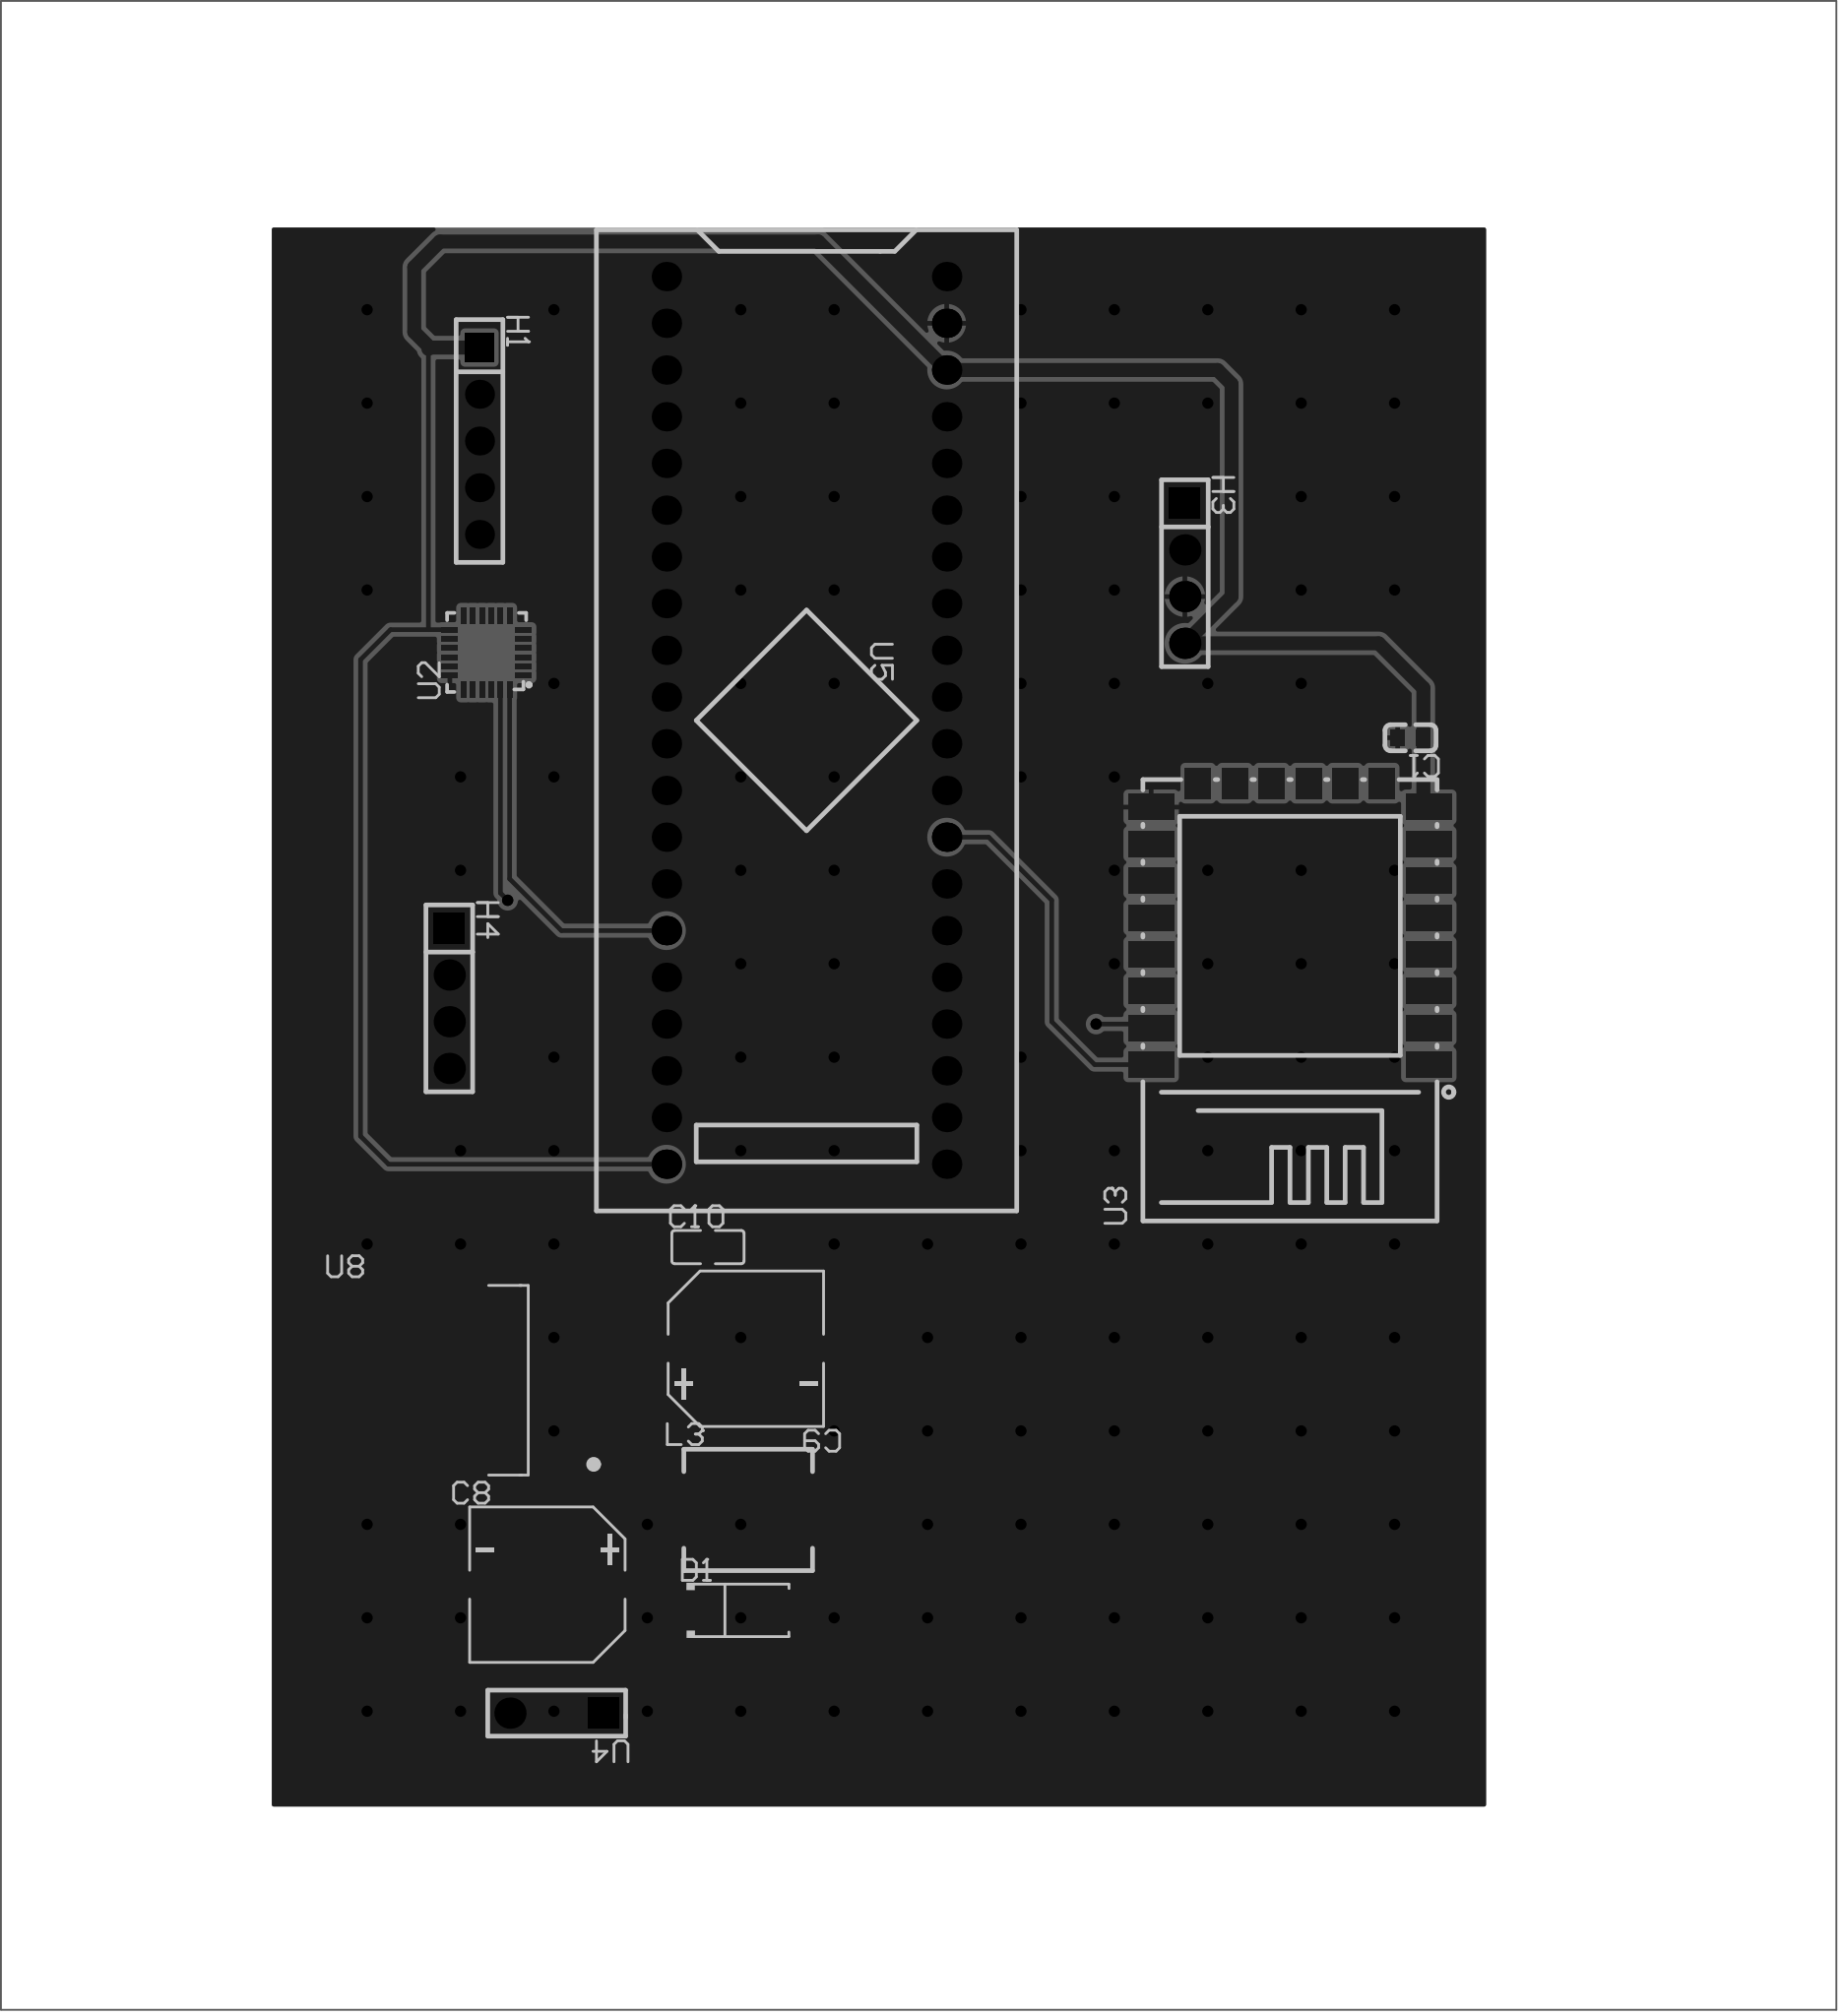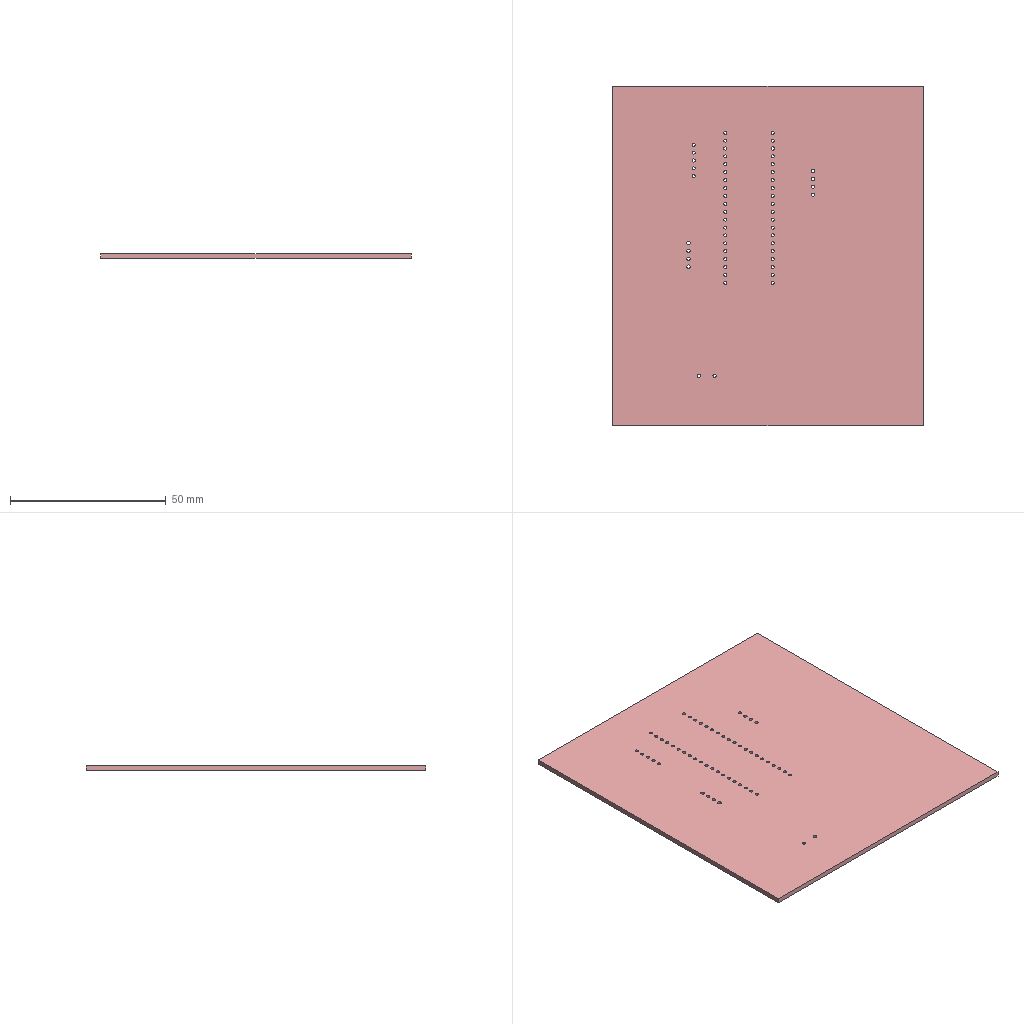Circuit board layout | Altium Designer | box 99.8 x 109.2 x 1.6 mm
Layer stack:
# Altium Designer layer stack of  (unit mm; dielectric type: 0 none, 1 core, 2 prepreg, 3 surface material)
index,name,kind,layer,copper_thickness_mm,dielectric_type,dielectric_thickness_mm,dielectric_material,dielectric_constant
0,Top Paste Mask Layer,other,,,,,,
1,Top Silkscreen Layer,other,,,,,,
2,Top Solder Mask Layer,dielectric,,,3,0.01,,3.3
3,Top Layer,copper,Top Layer,0.035,,,,
4,Dielectric1,dielectric,,,3,1.51,FR4,4.5
5,Bottom Layer,copper,Bottom Layer,0.035,,,,
6,Bottom Solder Mask Layer,dielectric,,,3,0.01,,3.3
7,Bottom Silkscreen Layer,other,,,,,,
8,Bottom Paste Mask Layer,other,,,,,,
# drill layer pairs: low layer,high layer
drill_pair,Top Layer,Bottom Layer
Part placement:
Designator,Comment,Layer,Footprint,Center-X(mm),Center-Y(mm),Rotation
C8,,TopLayer,CAP-SMD_BD8.0-L8.3-W8.3-RD,99.568,92.964,0
C9,,TopLayer,CAP-SMD_BD8.0-L8.3-W8.3-RD,110.363,105.791,180
C10,,TopLayer,C0805,108.302,111.317,0
D1,,TopLayer,SMA_L4.3-W2.6-LS5.2-RD,110.109,91.567,0
H3,Encoder,TopLayer,HDR-TH_4P-P2.54-V-M,134.239,147.955,270
H4,Servo,TopLayer,HDR-TH_4P-P2.54-V-M,94.234,124.841,270
L3,,TopLayer,IND-SMD_L7.0-W6.6,110.49,97.028,0
U2,MPU6050,TopLayer,QFN-24_L4.0-W4.0-P0.50-BL,96.266,143.637,90
U3,ESP8266,TopLayer,WIFIM-SMD_ESP-12F-ESP8266MOD,139.955,128.89,90
U4,5.08-2PIN straight header,TopLayer,HDR-TH_2P-P5.08_C9900004333,100.076,85.979,180
U8,LM2596S-5.0,TopLayer,TO-263-5_L10.2-W8.9-P1.70-BR,97.029,104.078,0
C1,10uF,TopLayer,C0603,146.511,139.01,180
U5,STM32F103C8T6-Card,TopLayer,CONN-TH_L53.3-W22.9_STM32F103C8T6-CARD,113.665,139.954,270
H1,,TopLayer,HDR-TH_5P-P2.54-V-F,95.879,155.144,270
Pad and via stacks:
# Altium Designer via and pad stacks of  (unit mm). Each distinct definition once, with the count of objects using it.
# via: kind,start_layer,end_layer,hole_mm,diameter_mm,mode(0 simple;1 top-mid-bottom;2 full stack),diameter_per_layer,count,example_net
# pad: kind,layer,hole_mm,hole_type(0 round;1 square;2 slot),plating,top_size,top_shape(1 round;2 rect;3 octagon;9 rounded rect),mid_size,bottom_size,mode,footprint,size_per_layer,count,example
pad,Top Layer,0,0,plated,3.61x1.26,2,3.61x1.26,3.61x1.26,0,CAP-SMD_BD8.0-L8.3-W8.3-RD,,4,C8.1
pad,Top Layer,0,0,plated,1.41x1.35,2,1.41x1.35,1.41x1.35,0,C0805,,2,C10.2
pad,Top Layer,0,0,plated,2x2,2,2x2,2x2,0,SMA_L4.3-W2.6-LS5.2-RD,,2,D1.2
pad,Top Layer,0,0,plated,2.799x3.701,2,2.799x3.701,2.799x3.701,0,IND-SMD_L7.0-W6.6,,2,L3.1
pad,Top Layer,0,0,plated,0.3x0.9,2,0.3x0.9,0.3x0.9,0,QFN-24_L4.0-W4.0-P0.50-BL,,24,U2.1
pad,Top Layer,0,0,plated,2.5x1.4,2,2.5x1.4,2.5x1.4,0,WIFIM-SMD_ESP-12F-ESP8266MOD,,16,U3.16
pad,Top Layer,0,0,plated,1.7x1.4,2,1.7x1.4,1.7x1.4,0,WIFIM-SMD_ESP-12F-ESP8266MOD,,6,U3.22
pad,Top Layer,0,0,plated,3.083x1.02,2,3.083x1.02,3.083x1.02,0,TO-263-5_L10.2-W8.9-P1.70-BR,,5,U8.1
pad,Top Layer,0,0,plated,8.5x11,2,8.5x11,8.5x11,0,TO-263-5_L10.2-W8.9-P1.70-BR,,1,U8.6
pad,Top Layer,0,0,plated,0.8x0.9,2,0.8x0.9,0.8x0.9,0,C0603,,2,C1.2
pad,Multi-Layer,1.1,0,plated,1.7x1.7,2,1.7x1.7,1.7x1.7,0,HDR-TH_4P-P2.54-V-M,,2,H3.1
pad,Multi-Layer,1.1,0,plated,1.7x1.7,1,1.7x1.7,1.7x1.7,0,HDR-TH_4P-P2.54-V-M,,6,H3.2
pad,Multi-Layer,1.1,0,plated,1.7x1.7,2,1.7x1.7,1.7x1.7,0,HDR-TH_2P-P5.08_C9900004333,,1,U4.1
pad,Multi-Layer,1.1,0,plated,1.7x1.7,1,1.7x1.7,1.7x1.7,0,HDR-TH_2P-P5.08_C9900004333,,1,U4.2
pad,Multi-Layer,1,0,plated,1.6x1.6,1,1.6x1.6,1.6x1.6,0,CONN-TH_L53.3-W22.9_STM32F103C8T6-CARD,,40,U5.1
pad,Multi-Layer,1.02,0,plated,1.575x1.575,1,1.575x1.575,1.575x1.575,0,HDR-TH_5P-P2.54-V-F,,4,H1.5
pad,Multi-Layer,1.02,0,plated,1.575x1.575,2,1.575x1.575,1.575x1.575,0,HDR-TH_5P-P2.54-V-F,,1,H1.1
via,Top Layer,Bottom Layer,0.3048,0.61,0,,134,MPU60501
Copper pours:
name,layer,net,type(0 solid;1 hatched;2 none)
Top Layer-GND,Top Layer,GND,0
Bottom Layer-GND,Bottom Layer,GND,0